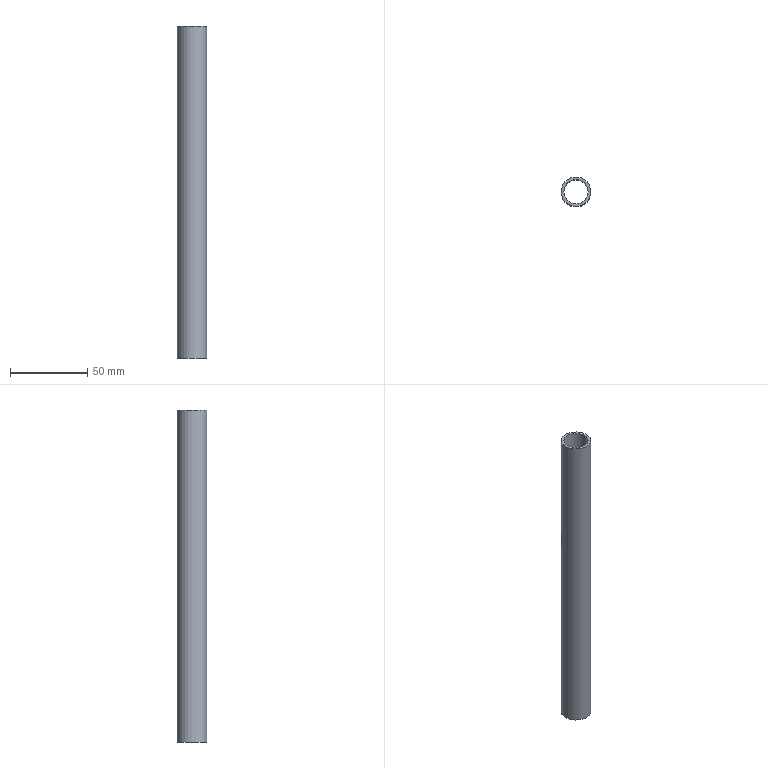Part | NX | features MG0322 rod 2 | 1 solid | 4 faces | box 19.05 x 19.05 x 215 mm | volume 19403 mm3 | cylinder 2 | plane 2 | commonest cylinder face diameters 15.748 x1 19.05 x1
STEP:
#1=CARTESIAN_POINT('',(9.525,0.,-200.025));
#2=VERTEX_POINT('',#1);
#3=CARTESIAN_POINT('',(0.,0.,-200.025));
#4=DIRECTION('',(0.,0.,1.));
#5=DIRECTION('',(1.,0.,0.));
#6=AXIS2_PLACEMENT_3D('',#3,#4,#5);
#7=CIRCLE('',#6,9.525);
#8=EDGE_CURVE('',#2,#2,#7,.T.);
#9=ORIENTED_EDGE('',*,*,#8,.T.);
#10=EDGE_LOOP('',(#9));
#11=FACE_BOUND('',#10,.T.);
#12=CARTESIAN_POINT('',(9.525,0.,14.975));
#13=VERTEX_POINT('',#12);
#14=CARTESIAN_POINT('',(0.,0.,14.975));
#15=DIRECTION('',(0.,0.,1.));
#16=DIRECTION('',(1.,0.,0.));
#17=AXIS2_PLACEMENT_3D('',#14,#15,#16);
#18=CIRCLE('',#17,9.525);
#19=EDGE_CURVE('',#13,#13,#18,.F.);
#20=ORIENTED_EDGE('',*,*,#19,.T.);
#21=EDGE_LOOP('',(#20));
#22=FACE_BOUND('',#21,.T.);
#23=CARTESIAN_POINT('',(0.,0.,-200.025));
#24=DIRECTION('',(0.,0.,1.));
#25=DIRECTION('',(1.,0.,0.));
#26=AXIS2_PLACEMENT_3D('',#23,#24,#25);
#27=CYLINDRICAL_SURFACE('',#26,9.525);
#28=ADVANCED_FACE('',(#11,#22),#27,.T.);
#29=CARTESIAN_POINT('',(7.874,0.,-200.025));
#30=VERTEX_POINT('',#29);
#31=CARTESIAN_POINT('',(0.,0.,-200.025));
#32=DIRECTION('',(0.,0.,1.));
#33=DIRECTION('',(1.,0.,0.));
#34=AXIS2_PLACEMENT_3D('',#31,#32,#33);
#35=CIRCLE('',#34,7.874);
#36=EDGE_CURVE('',#30,#30,#35,.T.);
#37=ORIENTED_EDGE('',*,*,#36,.F.);
#38=EDGE_LOOP('',(#37));
#39=FACE_BOUND('',#38,.T.);
#40=CARTESIAN_POINT('',(7.874,0.,14.975));
#41=VERTEX_POINT('',#40);
#42=CARTESIAN_POINT('',(0.,0.,14.975));
#43=DIRECTION('',(0.,0.,1.));
#44=DIRECTION('',(1.,0.,0.));
#45=AXIS2_PLACEMENT_3D('',#42,#43,#44);
#46=CIRCLE('',#45,7.874);
#47=EDGE_CURVE('',#41,#41,#46,.F.);
#48=ORIENTED_EDGE('',*,*,#47,.F.);
#49=EDGE_LOOP('',(#48));
#50=FACE_BOUND('',#49,.T.);
#51=CARTESIAN_POINT('',(0.,0.,-200.025));
#52=DIRECTION('',(0.,0.,1.));
#53=DIRECTION('',(1.,0.,0.));
#54=AXIS2_PLACEMENT_3D('',#51,#52,#53);
#55=CYLINDRICAL_SURFACE('',#54,7.874);
#56=ADVANCED_FACE('',(#39,#50),#55,.F.);
#57=ORIENTED_EDGE('',*,*,#36,.T.);
#58=EDGE_LOOP('',(#57));
#59=FACE_BOUND('',#58,.T.);
#60=ORIENTED_EDGE('',*,*,#8,.F.);
#61=EDGE_LOOP('',(#60));
#62=FACE_BOUND('',#61,.T.);
#63=CARTESIAN_POINT('',(0.,0.,-200.025));
#64=DIRECTION('',(0.,0.,1.));
#65=DIRECTION('',(1.,0.,0.));
#66=AXIS2_PLACEMENT_3D('',#63,#64,#65);
#67=PLANE('',#66);
#68=ADVANCED_FACE('',(#59,#62),#67,.F.);
#69=ORIENTED_EDGE('',*,*,#19,.F.);
#70=EDGE_LOOP('',(#69));
#71=FACE_BOUND('',#70,.T.);
#72=ORIENTED_EDGE('',*,*,#47,.T.);
#73=EDGE_LOOP('',(#72));
#74=FACE_BOUND('',#73,.T.);
#75=CARTESIAN_POINT('',(0.,0.,14.975));
#76=DIRECTION('',(0.,0.,1.));
#77=DIRECTION('',(1.,0.,0.));
#78=AXIS2_PLACEMENT_3D('',#75,#76,#77);
#79=PLANE('',#78);
#80=ADVANCED_FACE('',(#71,#74),#79,.T.);
#81=CLOSED_SHELL('',(#28,#56,#68,#80));
#82=MANIFOLD_SOLID_BREP('',#81);
#83=(LENGTH_UNIT()NAMED_UNIT(*)SI_UNIT(.MILLI.,.METRE.));
#84=UNCERTAINTY_MEASURE_WITH_UNIT(LENGTH_MEASURE(0.00001),#83,'','');
#85=(NAMED_UNIT(*)PLANE_ANGLE_UNIT()SI_UNIT($,.RADIAN.));
#86=(NAMED_UNIT(*)SI_UNIT($,.STERADIAN.)SOLID_ANGLE_UNIT());
#87=(GEOMETRIC_REPRESENTATION_CONTEXT(3)GLOBAL_UNCERTAINTY_ASSIGNED_CONTEXT((#84))GLOBAL_UNIT_ASSIGNED_CONTEXT((#83,#85,#86))REPRESENTATION_CONTEXT('',''));
#88=ADVANCED_BREP_SHAPE_REPRESENTATION('',(#82),#87);